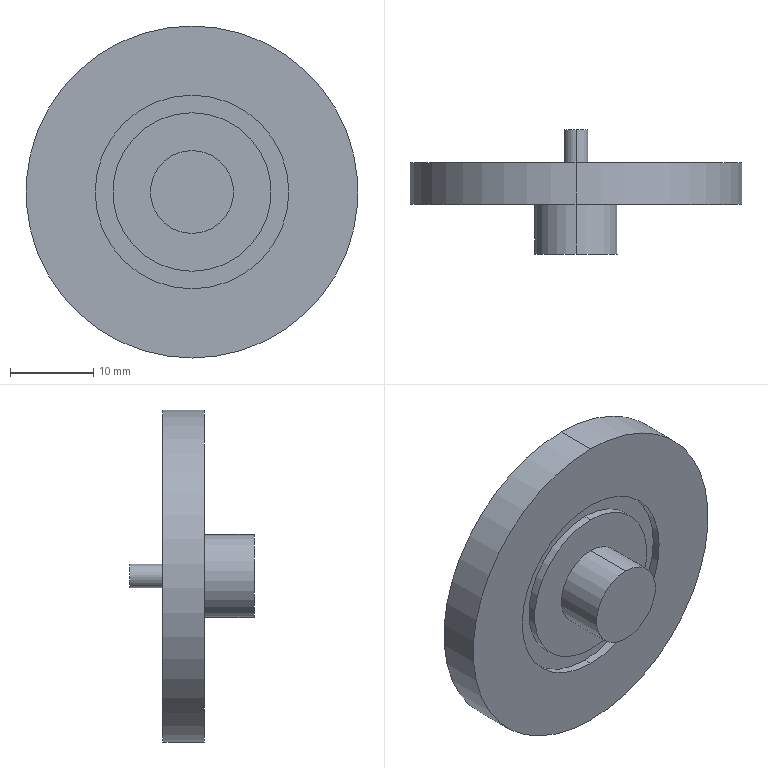Part | SolidWorks | features ICE 5, Extrusion 1 | 1 solid | 28 faces | box 40 x 15 x 40 mm | volume 6357 mm3 | cylinder 18 | plane 10 | commonest cylinder face diameters 2.85 x2 10 x2 16.818 x2 19.091 x2 20.068 x2 23.339 x2
STEP:
#1=CARTESIAN_POINT('',(0.,9.,1.425));
#2=VERTEX_POINT('',#1);
#3=CARTESIAN_POINT('',(0.,9.,-1.425));
#4=VERTEX_POINT('',#3);
#5=CARTESIAN_POINT('',(0.,9.,0.));
#6=DIRECTION('',(0.,1.,0.));
#7=DIRECTION('',(0.,0.,1.));
#8=AXIS2_PLACEMENT_3D('',#5,#6,#7);
#9=CIRCLE('',#8,1.425);
#10=EDGE_CURVE('',#2,#4,#9,.T.);
#11=ORIENTED_EDGE('',*,*,#10,.F.);
#12=CARTESIAN_POINT('',(0.,5.,1.425));
#13=VERTEX_POINT('',#12);
#14=CARTESIAN_POINT('',(0.,9.,1.425));
#15=DIRECTION('',(0.,-1.,0.));
#16=VECTOR('',#15,1000.);
#17=LINE('',#14,#16);
#18=EDGE_CURVE('',#2,#13,#17,.T.);
#19=ORIENTED_EDGE('',*,*,#18,.T.);
#20=CARTESIAN_POINT('',(0.,5.,-1.425));
#21=VERTEX_POINT('',#20);
#22=CARTESIAN_POINT('',(0.,5.,0.));
#23=DIRECTION('',(0.,1.,0.));
#24=DIRECTION('',(0.,0.,1.));
#25=AXIS2_PLACEMENT_3D('',#22,#23,#24);
#26=CIRCLE('',#25,1.425);
#27=EDGE_CURVE('',#13,#21,#26,.T.);
#28=ORIENTED_EDGE('',*,*,#27,.T.);
#29=CARTESIAN_POINT('',(0.,9.,-1.425));
#30=DIRECTION('',(0.,-1.,0.));
#31=VECTOR('',#30,1000.);
#32=LINE('',#29,#31);
#33=EDGE_CURVE('',#4,#21,#32,.T.);
#34=ORIENTED_EDGE('',*,*,#33,.F.);
#35=EDGE_LOOP('',(#11,#19,#28,#34));
#36=FACE_OUTER_BOUND('',#35,.T.);
#37=CARTESIAN_POINT('',(0.,9.,0.));
#38=DIRECTION('',(0.,-1.,0.));
#39=DIRECTION('',(0.,0.,-1.));
#40=AXIS2_PLACEMENT_3D('',#37,#38,#39);
#41=CYLINDRICAL_SURFACE('',#40,1.425);
#42=ADVANCED_FACE('',(#36),#41,.T.);
#43=CARTESIAN_POINT('',(0.,4.,8.409));
#44=VERTEX_POINT('',#43);
#45=CARTESIAN_POINT('',(0.,4.,-8.409));
#46=VERTEX_POINT('',#45);
#47=CARTESIAN_POINT('',(0.,4.,0.));
#48=DIRECTION('',(0.,1.,0.));
#49=DIRECTION('',(0.,0.,1.));
#50=AXIS2_PLACEMENT_3D('',#47,#48,#49);
#51=CIRCLE('',#50,8.409);
#52=EDGE_CURVE('',#44,#46,#51,.T.);
#53=ORIENTED_EDGE('',*,*,#52,.T.);
#54=CARTESIAN_POINT('',(0.,5.,-8.409));
#55=VERTEX_POINT('',#54);
#56=CARTESIAN_POINT('',(0.,4.,-8.409));
#57=DIRECTION('',(0.,1.,0.));
#58=VECTOR('',#57,1000.);
#59=LINE('',#56,#58);
#60=EDGE_CURVE('',#46,#55,#59,.T.);
#61=ORIENTED_EDGE('',*,*,#60,.T.);
#62=CARTESIAN_POINT('',(0.,5.,8.409));
#63=VERTEX_POINT('',#62);
#64=CARTESIAN_POINT('',(0.,5.,0.));
#65=DIRECTION('',(0.,1.,0.));
#66=DIRECTION('',(0.,0.,1.));
#67=AXIS2_PLACEMENT_3D('',#64,#65,#66);
#68=CIRCLE('',#67,8.409);
#69=EDGE_CURVE('',#63,#55,#68,.T.);
#70=ORIENTED_EDGE('',*,*,#69,.F.);
#71=CARTESIAN_POINT('',(0.,4.,8.409));
#72=DIRECTION('',(0.,1.,0.));
#73=VECTOR('',#72,1000.);
#74=LINE('',#71,#73);
#75=EDGE_CURVE('',#44,#63,#74,.T.);
#76=ORIENTED_EDGE('',*,*,#75,.F.);
#77=EDGE_LOOP('',(#53,#61,#70,#76));
#78=FACE_OUTER_BOUND('',#77,.T.);
#79=CARTESIAN_POINT('',(0.,4.,0.));
#80=DIRECTION('',(0.,1.,0.));
#81=DIRECTION('',(0.,0.,1.));
#82=AXIS2_PLACEMENT_3D('',#79,#80,#81);
#83=CYLINDRICAL_SURFACE('',#82,8.409);
#84=ADVANCED_FACE('',(#78),#83,.T.);
#85=CARTESIAN_POINT('',(0.,4.,-10.034));
#86=VERTEX_POINT('',#85);
#87=CARTESIAN_POINT('',(0.,4.,10.034));
#88=VERTEX_POINT('',#87);
#89=CARTESIAN_POINT('',(0.,4.,0.));
#90=DIRECTION('',(0.,1.,0.));
#91=DIRECTION('',(0.,0.,1.));
#92=AXIS2_PLACEMENT_3D('',#89,#90,#91);
#93=CIRCLE('',#92,10.034);
#94=EDGE_CURVE('',#86,#88,#93,.T.);
#95=ORIENTED_EDGE('',*,*,#94,.F.);
#96=CARTESIAN_POINT('',(0.,5.,-10.034));
#97=VERTEX_POINT('',#96);
#98=CARTESIAN_POINT('',(0.,4.,-10.034));
#99=DIRECTION('',(0.,1.,0.));
#100=VECTOR('',#99,1000.);
#101=LINE('',#98,#100);
#102=EDGE_CURVE('',#86,#97,#101,.T.);
#103=ORIENTED_EDGE('',*,*,#102,.T.);
#104=CARTESIAN_POINT('',(0.,5.,10.034));
#105=VERTEX_POINT('',#104);
#106=CARTESIAN_POINT('',(0.,5.,0.));
#107=DIRECTION('',(0.,1.,0.));
#108=DIRECTION('',(0.,0.,1.));
#109=AXIS2_PLACEMENT_3D('',#106,#107,#108);
#110=CIRCLE('',#109,10.034);
#111=EDGE_CURVE('',#97,#105,#110,.T.);
#112=ORIENTED_EDGE('',*,*,#111,.T.);
#113=CARTESIAN_POINT('',(0.,4.,10.034));
#114=DIRECTION('',(0.,1.,0.));
#115=VECTOR('',#114,1000.);
#116=LINE('',#113,#115);
#117=EDGE_CURVE('',#88,#105,#116,.T.);
#118=ORIENTED_EDGE('',*,*,#117,.F.);
#119=EDGE_LOOP('',(#95,#103,#112,#118));
#120=FACE_OUTER_BOUND('',#119,.T.);
#121=CARTESIAN_POINT('',(0.,4.,0.));
#122=DIRECTION('',(0.,1.,0.));
#123=DIRECTION('',(0.,0.,1.));
#124=AXIS2_PLACEMENT_3D('',#121,#122,#123);
#125=CYLINDRICAL_SURFACE('',#124,10.034);
#126=ADVANCED_FACE('',(#120),#125,.F.);
#127=CARTESIAN_POINT('',(0.,4.,15.634));
#128=VERTEX_POINT('',#127);
#129=CARTESIAN_POINT('',(0.,4.,-15.634));
#130=VERTEX_POINT('',#129);
#131=CARTESIAN_POINT('',(0.,4.,0.));
#132=DIRECTION('',(0.,1.,0.));
#133=DIRECTION('',(0.,0.,1.));
#134=AXIS2_PLACEMENT_3D('',#131,#132,#133);
#135=CIRCLE('',#134,15.634);
#136=EDGE_CURVE('',#128,#130,#135,.T.);
#137=ORIENTED_EDGE('',*,*,#136,.T.);
#138=CARTESIAN_POINT('',(0.,5.,-15.634));
#139=VERTEX_POINT('',#138);
#140=CARTESIAN_POINT('',(0.,4.,-15.634));
#141=DIRECTION('',(0.,1.,0.));
#142=VECTOR('',#141,1000.);
#143=LINE('',#140,#142);
#144=EDGE_CURVE('',#130,#139,#143,.T.);
#145=ORIENTED_EDGE('',*,*,#144,.T.);
#146=CARTESIAN_POINT('',(0.,5.,15.634));
#147=VERTEX_POINT('',#146);
#148=CARTESIAN_POINT('',(0.,5.,0.));
#149=DIRECTION('',(0.,1.,0.));
#150=DIRECTION('',(0.,0.,1.));
#151=AXIS2_PLACEMENT_3D('',#148,#149,#150);
#152=CIRCLE('',#151,15.634);
#153=EDGE_CURVE('',#147,#139,#152,.T.);
#154=ORIENTED_EDGE('',*,*,#153,.F.);
#155=CARTESIAN_POINT('',(0.,4.,15.634));
#156=DIRECTION('',(0.,1.,0.));
#157=VECTOR('',#156,1000.);
#158=LINE('',#155,#157);
#159=EDGE_CURVE('',#128,#147,#158,.T.);
#160=ORIENTED_EDGE('',*,*,#159,.F.);
#161=EDGE_LOOP('',(#137,#145,#154,#160));
#162=FACE_OUTER_BOUND('',#161,.T.);
#163=CARTESIAN_POINT('',(0.,4.,0.));
#164=DIRECTION('',(0.,1.,0.));
#165=DIRECTION('',(0.,0.,1.));
#166=AXIS2_PLACEMENT_3D('',#163,#164,#165);
#167=CYLINDRICAL_SURFACE('',#166,15.634);
#168=ADVANCED_FACE('',(#162),#167,.T.);
#169=CARTESIAN_POINT('',(0.,4.,-17.435));
#170=VERTEX_POINT('',#169);
#171=CARTESIAN_POINT('',(0.,4.,17.435));
#172=VERTEX_POINT('',#171);
#173=CARTESIAN_POINT('',(0.,4.,0.));
#174=DIRECTION('',(0.,1.,0.));
#175=DIRECTION('',(0.,0.,1.));
#176=AXIS2_PLACEMENT_3D('',#173,#174,#175);
#177=CIRCLE('',#176,17.435);
#178=EDGE_CURVE('',#170,#172,#177,.T.);
#179=ORIENTED_EDGE('',*,*,#178,.F.);
#180=CARTESIAN_POINT('',(0.,5.,-17.435));
#181=VERTEX_POINT('',#180);
#182=CARTESIAN_POINT('',(0.,4.,-17.435));
#183=DIRECTION('',(0.,1.,0.));
#184=VECTOR('',#183,1000.);
#185=LINE('',#182,#184);
#186=EDGE_CURVE('',#170,#181,#185,.T.);
#187=ORIENTED_EDGE('',*,*,#186,.T.);
#188=CARTESIAN_POINT('',(0.,5.,17.435));
#189=VERTEX_POINT('',#188);
#190=CARTESIAN_POINT('',(0.,5.,0.));
#191=DIRECTION('',(0.,1.,0.));
#192=DIRECTION('',(0.,0.,1.));
#193=AXIS2_PLACEMENT_3D('',#190,#191,#192);
#194=CIRCLE('',#193,17.435);
#195=EDGE_CURVE('',#181,#189,#194,.T.);
#196=ORIENTED_EDGE('',*,*,#195,.T.);
#197=CARTESIAN_POINT('',(0.,4.,17.435));
#198=DIRECTION('',(0.,1.,0.));
#199=VECTOR('',#198,1000.);
#200=LINE('',#197,#199);
#201=EDGE_CURVE('',#172,#189,#200,.T.);
#202=ORIENTED_EDGE('',*,*,#201,.F.);
#203=EDGE_LOOP('',(#179,#187,#196,#202));
#204=FACE_OUTER_BOUND('',#203,.T.);
#205=CARTESIAN_POINT('',(0.,4.,0.));
#206=DIRECTION('',(0.,1.,0.));
#207=DIRECTION('',(0.,0.,1.));
#208=AXIS2_PLACEMENT_3D('',#205,#206,#207);
#209=CYLINDRICAL_SURFACE('',#208,17.435);
#210=ADVANCED_FACE('',(#204),#209,.F.);
#211=CARTESIAN_POINT('',(0.,-6.,-5.));
#212=VERTEX_POINT('',#211);
#213=CARTESIAN_POINT('',(0.,-6.,5.));
#214=VERTEX_POINT('',#213);
#215=CARTESIAN_POINT('',(0.,-6.,0.));
#216=DIRECTION('',(0.,-1.,0.));
#217=DIRECTION('',(0.,0.,-1.));
#218=AXIS2_PLACEMENT_3D('',#215,#216,#217);
#219=CIRCLE('',#218,5.);
#220=EDGE_CURVE('',#212,#214,#219,.T.);
#221=ORIENTED_EDGE('',*,*,#220,.F.);
#222=CARTESIAN_POINT('',(0.,0.,-5.));
#223=VERTEX_POINT('',#222);
#224=CARTESIAN_POINT('',(0.,-6.,-5.));
#225=DIRECTION('',(0.,1.,0.));
#226=VECTOR('',#225,1000.);
#227=LINE('',#224,#226);
#228=EDGE_CURVE('',#212,#223,#227,.T.);
#229=ORIENTED_EDGE('',*,*,#228,.T.);
#230=CARTESIAN_POINT('',(0.,0.,5.));
#231=VERTEX_POINT('',#230);
#232=CARTESIAN_POINT('',(0.,0.,0.));
#233=DIRECTION('',(0.,-1.,0.));
#234=DIRECTION('',(0.,0.,-1.));
#235=AXIS2_PLACEMENT_3D('',#232,#233,#234);
#236=CIRCLE('',#235,5.);
#237=EDGE_CURVE('',#223,#231,#236,.T.);
#238=ORIENTED_EDGE('',*,*,#237,.T.);
#239=CARTESIAN_POINT('',(0.,-6.,5.));
#240=DIRECTION('',(0.,1.,0.));
#241=VECTOR('',#240,1000.);
#242=LINE('',#239,#241);
#243=EDGE_CURVE('',#214,#231,#242,.T.);
#244=ORIENTED_EDGE('',*,*,#243,.F.);
#245=EDGE_LOOP('',(#221,#229,#238,#244));
#246=FACE_OUTER_BOUND('',#245,.T.);
#247=CARTESIAN_POINT('',(0.,-6.,0.));
#248=DIRECTION('',(0.,1.,0.));
#249=DIRECTION('',(0.,0.,1.));
#250=AXIS2_PLACEMENT_3D('',#247,#248,#249);
#251=CYLINDRICAL_SURFACE('',#250,5.);
#252=ADVANCED_FACE('',(#246),#251,.T.);
#253=CARTESIAN_POINT('',(0.,1.,-9.545));
#254=VERTEX_POINT('',#253);
#255=CARTESIAN_POINT('',(0.,1.,9.545));
#256=VERTEX_POINT('',#255);
#257=CARTESIAN_POINT('',(0.,1.,0.));
#258=DIRECTION('',(0.,-1.,0.));
#259=DIRECTION('',(0.,0.,-1.));
#260=AXIS2_PLACEMENT_3D('',#257,#258,#259);
#261=CIRCLE('',#260,9.545);
#262=EDGE_CURVE('',#254,#256,#261,.T.);
#263=ORIENTED_EDGE('',*,*,#262,.T.);
#264=CARTESIAN_POINT('',(0.,0.,9.545));
#265=VERTEX_POINT('',#264);
#266=CARTESIAN_POINT('',(0.,1.,9.545));
#267=DIRECTION('',(0.,-1.,0.));
#268=VECTOR('',#267,1000.);
#269=LINE('',#266,#268);
#270=EDGE_CURVE('',#256,#265,#269,.T.);
#271=ORIENTED_EDGE('',*,*,#270,.T.);
#272=CARTESIAN_POINT('',(0.,0.,-9.545));
#273=VERTEX_POINT('',#272);
#274=CARTESIAN_POINT('',(0.,0.,0.));
#275=DIRECTION('',(0.,-1.,0.));
#276=DIRECTION('',(0.,0.,-1.));
#277=AXIS2_PLACEMENT_3D('',#274,#275,#276);
#278=CIRCLE('',#277,9.545);
#279=EDGE_CURVE('',#273,#265,#278,.T.);
#280=ORIENTED_EDGE('',*,*,#279,.F.);
#281=CARTESIAN_POINT('',(0.,1.,-9.545));
#282=DIRECTION('',(0.,-1.,0.));
#283=VECTOR('',#282,1000.);
#284=LINE('',#281,#283);
#285=EDGE_CURVE('',#254,#273,#284,.T.);
#286=ORIENTED_EDGE('',*,*,#285,.F.);
#287=EDGE_LOOP('',(#263,#271,#280,#286));
#288=FACE_OUTER_BOUND('',#287,.T.);
#289=CARTESIAN_POINT('',(0.,1.,0.));
#290=DIRECTION('',(0.,-1.,0.));
#291=DIRECTION('',(0.,0.,-1.));
#292=AXIS2_PLACEMENT_3D('',#289,#290,#291);
#293=CYLINDRICAL_SURFACE('',#292,9.545);
#294=ADVANCED_FACE('',(#288),#293,.T.);
#295=CARTESIAN_POINT('',(0.,1.,11.669));
#296=VERTEX_POINT('',#295);
#297=CARTESIAN_POINT('',(0.,1.,-11.669));
#298=VERTEX_POINT('',#297);
#299=CARTESIAN_POINT('',(0.,1.,0.));
#300=DIRECTION('',(0.,-1.,0.));
#301=DIRECTION('',(0.,0.,-1.));
#302=AXIS2_PLACEMENT_3D('',#299,#300,#301);
#303=CIRCLE('',#302,11.669);
#304=EDGE_CURVE('',#296,#298,#303,.T.);
#305=ORIENTED_EDGE('',*,*,#304,.F.);
#306=CARTESIAN_POINT('',(0.,0.,11.669));
#307=VERTEX_POINT('',#306);
#308=CARTESIAN_POINT('',(0.,1.,11.669));
#309=DIRECTION('',(0.,-1.,0.));
#310=VECTOR('',#309,1000.);
#311=LINE('',#308,#310);
#312=EDGE_CURVE('',#296,#307,#311,.T.);
#313=ORIENTED_EDGE('',*,*,#312,.T.);
#314=CARTESIAN_POINT('',(0.,0.,-11.669));
#315=VERTEX_POINT('',#314);
#316=CARTESIAN_POINT('',(0.,0.,0.));
#317=DIRECTION('',(0.,-1.,0.));
#318=DIRECTION('',(0.,0.,-1.));
#319=AXIS2_PLACEMENT_3D('',#316,#317,#318);
#320=CIRCLE('',#319,11.669);
#321=EDGE_CURVE('',#307,#315,#320,.T.);
#322=ORIENTED_EDGE('',*,*,#321,.T.);
#323=CARTESIAN_POINT('',(0.,1.,-11.669));
#324=DIRECTION('',(0.,-1.,0.));
#325=VECTOR('',#324,1000.);
#326=LINE('',#323,#325);
#327=EDGE_CURVE('',#298,#315,#326,.T.);
#328=ORIENTED_EDGE('',*,*,#327,.F.);
#329=EDGE_LOOP('',(#305,#313,#322,#328));
#330=FACE_OUTER_BOUND('',#329,.T.);
#331=CARTESIAN_POINT('',(0.,1.,0.));
#332=DIRECTION('',(0.,-1.,0.));
#333=DIRECTION('',(0.,0.,-1.));
#334=AXIS2_PLACEMENT_3D('',#331,#332,#333);
#335=CYLINDRICAL_SURFACE('',#334,11.669);
#336=ADVANCED_FACE('',(#330),#335,.F.);
#337=CARTESIAN_POINT('',(0.,5.,20.));
#338=VERTEX_POINT('',#337);
#339=CARTESIAN_POINT('',(0.,5.,-20.));
#340=VERTEX_POINT('',#339);
#341=CARTESIAN_POINT('',(0.,5.,0.));
#342=DIRECTION('',(0.,1.,0.));
#343=DIRECTION('',(0.,0.,1.));
#344=AXIS2_PLACEMENT_3D('',#341,#342,#343);
#345=CIRCLE('',#344,20.);
#346=EDGE_CURVE('',#338,#340,#345,.T.);
#347=ORIENTED_EDGE('',*,*,#346,.F.);
#348=CARTESIAN_POINT('',(0.,0.,20.));
#349=VERTEX_POINT('',#348);
#350=CARTESIAN_POINT('',(0.,5.,20.));
#351=DIRECTION('',(0.,-1.,0.));
#352=VECTOR('',#351,1000.);
#353=LINE('',#350,#352);
#354=EDGE_CURVE('',#338,#349,#353,.T.);
#355=ORIENTED_EDGE('',*,*,#354,.T.);
#356=CARTESIAN_POINT('',(0.,0.,-20.));
#357=VERTEX_POINT('',#356);
#358=CARTESIAN_POINT('',(0.,0.,0.));
#359=DIRECTION('',(0.,1.,0.));
#360=DIRECTION('',(0.,0.,1.));
#361=AXIS2_PLACEMENT_3D('',#358,#359,#360);
#362=CIRCLE('',#361,20.);
#363=EDGE_CURVE('',#349,#357,#362,.T.);
#364=ORIENTED_EDGE('',*,*,#363,.T.);
#365=CARTESIAN_POINT('',(0.,5.,-20.));
#366=DIRECTION('',(0.,-1.,0.));
#367=VECTOR('',#366,1000.);
#368=LINE('',#365,#367);
#369=EDGE_CURVE('',#340,#357,#368,.T.);
#370=ORIENTED_EDGE('',*,*,#369,.F.);
#371=EDGE_LOOP('',(#347,#355,#364,#370));
#372=FACE_OUTER_BOUND('',#371,.T.);
#373=CARTESIAN_POINT('',(0.,5.,0.));
#374=DIRECTION('',(0.,-1.,0.));
#375=DIRECTION('',(0.,0.,-1.));
#376=AXIS2_PLACEMENT_3D('',#373,#374,#375);
#377=CYLINDRICAL_SURFACE('',#376,20.);
#378=ADVANCED_FACE('',(#372),#377,.T.);
#379=ORIENTED_EDGE('',*,*,#354,.F.);
#380=CARTESIAN_POINT('',(0.,5.,0.));
#381=DIRECTION('',(0.,1.,0.));
#382=DIRECTION('',(0.,0.,1.));
#383=AXIS2_PLACEMENT_3D('',#380,#381,#382);
#384=CIRCLE('',#383,20.);
#385=EDGE_CURVE('',#340,#338,#384,.T.);
#386=ORIENTED_EDGE('',*,*,#385,.F.);
#387=ORIENTED_EDGE('',*,*,#369,.T.);
#388=CARTESIAN_POINT('',(0.,0.,0.));
#389=DIRECTION('',(0.,1.,0.));
#390=DIRECTION('',(0.,0.,1.));
#391=AXIS2_PLACEMENT_3D('',#388,#389,#390);
#392=CIRCLE('',#391,20.);
#393=EDGE_CURVE('',#357,#349,#392,.T.);
#394=ORIENTED_EDGE('',*,*,#393,.T.);
#395=EDGE_LOOP('',(#379,#386,#387,#394));
#396=FACE_OUTER_BOUND('',#395,.T.);
#397=CARTESIAN_POINT('',(0.,5.,0.));
#398=DIRECTION('',(0.,-1.,0.));
#399=DIRECTION('',(0.,0.,-1.));
#400=AXIS2_PLACEMENT_3D('',#397,#398,#399);
#401=CYLINDRICAL_SURFACE('',#400,20.);
#402=ADVANCED_FACE('',(#396),#401,.T.);
#403=CARTESIAN_POINT('',(0.,5.,0.));
#404=DIRECTION('',(0.,1.,0.));
#405=DIRECTION('',(0.,0.,1.));
#406=AXIS2_PLACEMENT_3D('',#403,#404,#405);
#407=CIRCLE('',#406,17.435);
#408=EDGE_CURVE('',#189,#181,#407,.T.);
#409=ORIENTED_EDGE('',*,*,#408,.F.);
#410=ORIENTED_EDGE('',*,*,#195,.F.);
#411=EDGE_LOOP('',(#409,#410));
#412=FACE_BOUND('',#411,.T.);
#413=ORIENTED_EDGE('',*,*,#385,.T.);
#414=ORIENTED_EDGE('',*,*,#346,.T.);
#415=EDGE_LOOP('',(#413,#414));
#416=FACE_OUTER_BOUND('',#415,.T.);
#417=CARTESIAN_POINT('',(0.,5.,0.));
#418=DIRECTION('',(0.,1.,0.));
#419=DIRECTION('',(0.,0.,1.));
#420=AXIS2_PLACEMENT_3D('',#417,#418,#419);
#421=PLANE('',#420);
#422=ADVANCED_FACE('',(#412,#416),#421,.T.);
#423=CARTESIAN_POINT('',(0.,0.,0.));
#424=DIRECTION('',(0.,-1.,0.));
#425=DIRECTION('',(0.,0.,-1.));
#426=AXIS2_PLACEMENT_3D('',#423,#424,#425);
#427=CIRCLE('',#426,11.669);
#428=EDGE_CURVE('',#315,#307,#427,.T.);
#429=ORIENTED_EDGE('',*,*,#428,.F.);
#430=ORIENTED_EDGE('',*,*,#321,.F.);
#431=EDGE_LOOP('',(#429,#430));
#432=FACE_BOUND('',#431,.T.);
#433=ORIENTED_EDGE('',*,*,#393,.F.);
#434=ORIENTED_EDGE('',*,*,#363,.F.);
#435=EDGE_LOOP('',(#433,#434));
#436=FACE_OUTER_BOUND('',#435,.T.);
#437=CARTESIAN_POINT('',(0.,0.,0.));
#438=DIRECTION('',(0.,1.,0.));
#439=DIRECTION('',(0.,0.,1.));
#440=AXIS2_PLACEMENT_3D('',#437,#438,#439);
#441=PLANE('',#440);
#442=ADVANCED_FACE('',(#432,#436),#441,.F.);
#443=ORIENTED_EDGE('',*,*,#312,.F.);
#444=CARTESIAN_POINT('',(0.,1.,0.));
#445=DIRECTION('',(0.,-1.,0.));
#446=DIRECTION('',(0.,0.,-1.));
#447=AXIS2_PLACEMENT_3D('',#444,#445,#446);
#448=CIRCLE('',#447,11.669);
#449=EDGE_CURVE('',#298,#296,#448,.T.);
#450=ORIENTED_EDGE('',*,*,#449,.F.);
#451=ORIENTED_EDGE('',*,*,#327,.T.);
#452=ORIENTED_EDGE('',*,*,#428,.T.);
#453=EDGE_LOOP('',(#443,#450,#451,#452));
#454=FACE_OUTER_BOUND('',#453,.T.);
#455=CARTESIAN_POINT('',(0.,1.,0.));
#456=DIRECTION('',(0.,-1.,0.));
#457=DIRECTION('',(0.,0.,-1.));
#458=AXIS2_PLACEMENT_3D('',#455,#456,#457);
#459=CYLINDRICAL_SURFACE('',#458,11.669);
#460=ADVANCED_FACE('',(#454),#459,.F.);
#461=ORIENTED_EDGE('',*,*,#262,.F.);
#462=CARTESIAN_POINT('',(0.,1.,0.));
#463=DIRECTION('',(0.,-1.,0.));
#464=DIRECTION('',(0.,0.,-1.));
#465=AXIS2_PLACEMENT_3D('',#462,#463,#464);
#466=CIRCLE('',#465,9.545);
#467=EDGE_CURVE('',#256,#254,#466,.T.);
#468=ORIENTED_EDGE('',*,*,#467,.F.);
#469=EDGE_LOOP('',(#461,#468));
#470=FACE_BOUND('',#469,.T.);
#471=ORIENTED_EDGE('',*,*,#449,.T.);
#472=ORIENTED_EDGE('',*,*,#304,.T.);
#473=EDGE_LOOP('',(#471,#472));
#474=FACE_OUTER_BOUND('',#473,.T.);
#475=CARTESIAN_POINT('',(0.,1.,0.));
#476=DIRECTION('',(0.,-1.,0.));
#477=DIRECTION('',(0.,0.,-1.));
#478=AXIS2_PLACEMENT_3D('',#475,#476,#477);
#479=PLANE('',#478);
#480=ADVANCED_FACE('',(#470,#474),#479,.T.);
#481=ORIENTED_EDGE('',*,*,#270,.F.);
#482=ORIENTED_EDGE('',*,*,#467,.T.);
#483=ORIENTED_EDGE('',*,*,#285,.T.);
#484=CARTESIAN_POINT('',(0.,0.,0.));
#485=DIRECTION('',(0.,-1.,0.));
#486=DIRECTION('',(0.,0.,-1.));
#487=AXIS2_PLACEMENT_3D('',#484,#485,#486);
#488=CIRCLE('',#487,9.545);
#489=EDGE_CURVE('',#265,#273,#488,.T.);
#490=ORIENTED_EDGE('',*,*,#489,.F.);
#491=EDGE_LOOP('',(#481,#482,#483,#490));
#492=FACE_OUTER_BOUND('',#491,.T.);
#493=CARTESIAN_POINT('',(0.,1.,0.));
#494=DIRECTION('',(0.,-1.,0.));
#495=DIRECTION('',(0.,0.,-1.));
#496=AXIS2_PLACEMENT_3D('',#493,#494,#495);
#497=CYLINDRICAL_SURFACE('',#496,9.545);
#498=ADVANCED_FACE('',(#492),#497,.T.);
#499=CARTESIAN_POINT('',(0.,-6.,0.));
#500=DIRECTION('',(0.,-1.,0.));
#501=DIRECTION('',(0.,0.,-1.));
#502=AXIS2_PLACEMENT_3D('',#499,#500,#501);
#503=CIRCLE('',#502,5.);
#504=EDGE_CURVE('',#214,#212,#503,.T.);
#505=ORIENTED_EDGE('',*,*,#504,.T.);
#506=ORIENTED_EDGE('',*,*,#220,.T.);
#507=EDGE_LOOP('',(#505,#506));
#508=FACE_OUTER_BOUND('',#507,.T.);
#509=CARTESIAN_POINT('',(0.,-6.,0.));
#510=DIRECTION('',(0.,-1.,0.));
#511=DIRECTION('',(0.,0.,-1.));
#512=AXIS2_PLACEMENT_3D('',#509,#510,#511);
#513=PLANE('',#512);
#514=ADVANCED_FACE('',(#508),#513,.T.);
#515=ORIENTED_EDGE('',*,*,#228,.F.);
#516=ORIENTED_EDGE('',*,*,#504,.F.);
#517=ORIENTED_EDGE('',*,*,#243,.T.);
#518=CARTESIAN_POINT('',(0.,0.,0.));
#519=DIRECTION('',(0.,-1.,0.));
#520=DIRECTION('',(0.,0.,-1.));
#521=AXIS2_PLACEMENT_3D('',#518,#519,#520);
#522=CIRCLE('',#521,5.);
#523=EDGE_CURVE('',#231,#223,#522,.T.);
#524=ORIENTED_EDGE('',*,*,#523,.T.);
#525=EDGE_LOOP('',(#515,#516,#517,#524));
#526=FACE_OUTER_BOUND('',#525,.T.);
#527=CARTESIAN_POINT('',(0.,-6.,0.));
#528=DIRECTION('',(0.,1.,0.));
#529=DIRECTION('',(0.,0.,1.));
#530=AXIS2_PLACEMENT_3D('',#527,#528,#529);
#531=CYLINDRICAL_SURFACE('',#530,5.);
#532=ADVANCED_FACE('',(#526),#531,.T.);
#533=ORIENTED_EDGE('',*,*,#523,.F.);
#534=ORIENTED_EDGE('',*,*,#237,.F.);
#535=EDGE_LOOP('',(#533,#534));
#536=FACE_BOUND('',#535,.T.);
#537=ORIENTED_EDGE('',*,*,#279,.T.);
#538=ORIENTED_EDGE('',*,*,#489,.T.);
#539=EDGE_LOOP('',(#537,#538));
#540=FACE_OUTER_BOUND('',#539,.T.);
#541=CARTESIAN_POINT('',(0.,0.,0.));
#542=DIRECTION('',(0.,1.,0.));
#543=DIRECTION('',(0.,0.,1.));
#544=AXIS2_PLACEMENT_3D('',#541,#542,#543);
#545=PLANE('',#544);
#546=ADVANCED_FACE('',(#536,#540),#545,.F.);
#547=ORIENTED_EDGE('',*,*,#186,.F.);
#548=CARTESIAN_POINT('',(0.,4.,0.));
#549=DIRECTION('',(0.,1.,0.));
#550=DIRECTION('',(0.,0.,1.));
#551=AXIS2_PLACEMENT_3D('',#548,#549,#550);
#552=CIRCLE('',#551,17.435);
#553=EDGE_CURVE('',#172,#170,#552,.T.);
#554=ORIENTED_EDGE('',*,*,#553,.F.);
#555=ORIENTED_EDGE('',*,*,#201,.T.);
#556=ORIENTED_EDGE('',*,*,#408,.T.);
#557=EDGE_LOOP('',(#547,#554,#555,#556));
#558=FACE_OUTER_BOUND('',#557,.T.);
#559=CARTESIAN_POINT('',(0.,4.,0.));
#560=DIRECTION('',(0.,1.,0.));
#561=DIRECTION('',(0.,0.,1.));
#562=AXIS2_PLACEMENT_3D('',#559,#560,#561);
#563=CYLINDRICAL_SURFACE('',#562,17.435);
#564=ADVANCED_FACE('',(#558),#563,.F.);
#565=ORIENTED_EDGE('',*,*,#136,.F.);
#566=CARTESIAN_POINT('',(0.,4.,0.));
#567=DIRECTION('',(0.,1.,0.));
#568=DIRECTION('',(0.,0.,1.));
#569=AXIS2_PLACEMENT_3D('',#566,#567,#568);
#570=CIRCLE('',#569,15.634);
#571=EDGE_CURVE('',#130,#128,#570,.T.);
#572=ORIENTED_EDGE('',*,*,#571,.F.);
#573=EDGE_LOOP('',(#565,#572));
#574=FACE_BOUND('',#573,.T.);
#575=ORIENTED_EDGE('',*,*,#553,.T.);
#576=ORIENTED_EDGE('',*,*,#178,.T.);
#577=EDGE_LOOP('',(#575,#576));
#578=FACE_OUTER_BOUND('',#577,.T.);
#579=CARTESIAN_POINT('',(0.,4.,0.));
#580=DIRECTION('',(0.,1.,0.));
#581=DIRECTION('',(0.,0.,1.));
#582=AXIS2_PLACEMENT_3D('',#579,#580,#581);
#583=PLANE('',#582);
#584=ADVANCED_FACE('',(#574,#578),#583,.T.);
#585=ORIENTED_EDGE('',*,*,#144,.F.);
#586=ORIENTED_EDGE('',*,*,#571,.T.);
#587=ORIENTED_EDGE('',*,*,#159,.T.);
#588=CARTESIAN_POINT('',(0.,5.,0.));
#589=DIRECTION('',(0.,1.,0.));
#590=DIRECTION('',(0.,0.,1.));
#591=AXIS2_PLACEMENT_3D('',#588,#589,#590);
#592=CIRCLE('',#591,15.634);
#593=EDGE_CURVE('',#139,#147,#592,.T.);
#594=ORIENTED_EDGE('',*,*,#593,.F.);
#595=EDGE_LOOP('',(#585,#586,#587,#594));
#596=FACE_OUTER_BOUND('',#595,.T.);
#597=CARTESIAN_POINT('',(0.,4.,0.));
#598=DIRECTION('',(0.,1.,0.));
#599=DIRECTION('',(0.,0.,1.));
#600=AXIS2_PLACEMENT_3D('',#597,#598,#599);
#601=CYLINDRICAL_SURFACE('',#600,15.634);
#602=ADVANCED_FACE('',(#596),#601,.T.);
#603=CARTESIAN_POINT('',(0.,5.,0.));
#604=DIRECTION('',(0.,1.,0.));
#605=DIRECTION('',(0.,0.,1.));
#606=AXIS2_PLACEMENT_3D('',#603,#604,#605);
#607=CIRCLE('',#606,10.034);
#608=EDGE_CURVE('',#105,#97,#607,.T.);
#609=ORIENTED_EDGE('',*,*,#608,.F.);
#610=ORIENTED_EDGE('',*,*,#111,.F.);
#611=EDGE_LOOP('',(#609,#610));
#612=FACE_BOUND('',#611,.T.);
#613=ORIENTED_EDGE('',*,*,#153,.T.);
#614=ORIENTED_EDGE('',*,*,#593,.T.);
#615=EDGE_LOOP('',(#613,#614));
#616=FACE_OUTER_BOUND('',#615,.T.);
#617=CARTESIAN_POINT('',(0.,5.,0.));
#618=DIRECTION('',(0.,1.,0.));
#619=DIRECTION('',(0.,0.,1.));
#620=AXIS2_PLACEMENT_3D('',#617,#618,#619);
#621=PLANE('',#620);
#622=ADVANCED_FACE('',(#612,#616),#621,.T.);
#623=ORIENTED_EDGE('',*,*,#102,.F.);
#624=CARTESIAN_POINT('',(0.,4.,0.));
#625=DIRECTION('',(0.,1.,0.));
#626=DIRECTION('',(0.,0.,1.));
#627=AXIS2_PLACEMENT_3D('',#624,#625,#626);
#628=CIRCLE('',#627,10.034);
#629=EDGE_CURVE('',#88,#86,#628,.T.);
#630=ORIENTED_EDGE('',*,*,#629,.F.);
#631=ORIENTED_EDGE('',*,*,#117,.T.);
#632=ORIENTED_EDGE('',*,*,#608,.T.);
#633=EDGE_LOOP('',(#623,#630,#631,#632));
#634=FACE_OUTER_BOUND('',#633,.T.);
#635=CARTESIAN_POINT('',(0.,4.,0.));
#636=DIRECTION('',(0.,1.,0.));
#637=DIRECTION('',(0.,0.,1.));
#638=AXIS2_PLACEMENT_3D('',#635,#636,#637);
#639=CYLINDRICAL_SURFACE('',#638,10.034);
#640=ADVANCED_FACE('',(#634),#639,.F.);
#641=ORIENTED_EDGE('',*,*,#52,.F.);
#642=CARTESIAN_POINT('',(0.,4.,0.));
#643=DIRECTION('',(0.,1.,0.));
#644=DIRECTION('',(0.,0.,1.));
#645=AXIS2_PLACEMENT_3D('',#642,#643,#644);
#646=CIRCLE('',#645,8.409);
#647=EDGE_CURVE('',#46,#44,#646,.T.);
#648=ORIENTED_EDGE('',*,*,#647,.F.);
#649=EDGE_LOOP('',(#641,#648));
#650=FACE_BOUND('',#649,.T.);
#651=ORIENTED_EDGE('',*,*,#629,.T.);
#652=ORIENTED_EDGE('',*,*,#94,.T.);
#653=EDGE_LOOP('',(#651,#652));
#654=FACE_OUTER_BOUND('',#653,.T.);
#655=CARTESIAN_POINT('',(0.,4.,0.));
#656=DIRECTION('',(0.,1.,0.));
#657=DIRECTION('',(0.,0.,1.));
#658=AXIS2_PLACEMENT_3D('',#655,#656,#657);
#659=PLANE('',#658);
#660=ADVANCED_FACE('',(#650,#654),#659,.T.);
#661=ORIENTED_EDGE('',*,*,#60,.F.);
#662=ORIENTED_EDGE('',*,*,#647,.T.);
#663=ORIENTED_EDGE('',*,*,#75,.T.);
#664=CARTESIAN_POINT('',(0.,5.,0.));
#665=DIRECTION('',(0.,1.,0.));
#666=DIRECTION('',(0.,0.,1.));
#667=AXIS2_PLACEMENT_3D('',#664,#665,#666);
#668=CIRCLE('',#667,8.409);
#669=EDGE_CURVE('',#55,#63,#668,.T.);
#670=ORIENTED_EDGE('',*,*,#669,.F.);
#671=EDGE_LOOP('',(#661,#662,#663,#670));
#672=FACE_OUTER_BOUND('',#671,.T.);
#673=CARTESIAN_POINT('',(0.,4.,0.));
#674=DIRECTION('',(0.,1.,0.));
#675=DIRECTION('',(0.,0.,1.));
#676=AXIS2_PLACEMENT_3D('',#673,#674,#675);
#677=CYLINDRICAL_SURFACE('',#676,8.409);
#678=ADVANCED_FACE('',(#672),#677,.T.);
#679=CARTESIAN_POINT('',(0.,9.,0.));
#680=DIRECTION('',(0.,1.,0.));
#681=DIRECTION('',(0.,0.,1.));
#682=AXIS2_PLACEMENT_3D('',#679,#680,#681);
#683=CIRCLE('',#682,1.425);
#684=EDGE_CURVE('',#4,#2,#683,.T.);
#685=ORIENTED_EDGE('',*,*,#684,.T.);
#686=ORIENTED_EDGE('',*,*,#10,.T.);
#687=EDGE_LOOP('',(#685,#686));
#688=FACE_OUTER_BOUND('',#687,.T.);
#689=CARTESIAN_POINT('',(0.,9.,0.));
#690=DIRECTION('',(0.,1.,0.));
#691=DIRECTION('',(0.,0.,1.));
#692=AXIS2_PLACEMENT_3D('',#689,#690,#691);
#693=PLANE('',#692);
#694=ADVANCED_FACE('',(#688),#693,.T.);
#695=ORIENTED_EDGE('',*,*,#18,.F.);
#696=ORIENTED_EDGE('',*,*,#684,.F.);
#697=ORIENTED_EDGE('',*,*,#33,.T.);
#698=CARTESIAN_POINT('',(0.,5.,0.));
#699=DIRECTION('',(0.,1.,0.));
#700=DIRECTION('',(0.,0.,1.));
#701=AXIS2_PLACEMENT_3D('',#698,#699,#700);
#702=CIRCLE('',#701,1.425);
#703=EDGE_CURVE('',#21,#13,#702,.T.);
#704=ORIENTED_EDGE('',*,*,#703,.T.);
#705=EDGE_LOOP('',(#695,#696,#697,#704));
#706=FACE_OUTER_BOUND('',#705,.T.);
#707=CARTESIAN_POINT('',(0.,9.,0.));
#708=DIRECTION('',(0.,-1.,0.));
#709=DIRECTION('',(0.,0.,-1.));
#710=AXIS2_PLACEMENT_3D('',#707,#708,#709);
#711=CYLINDRICAL_SURFACE('',#710,1.425);
#712=ADVANCED_FACE('',(#706),#711,.T.);
#713=ORIENTED_EDGE('',*,*,#703,.F.);
#714=ORIENTED_EDGE('',*,*,#27,.F.);
#715=EDGE_LOOP('',(#713,#714));
#716=FACE_BOUND('',#715,.T.);
#717=ORIENTED_EDGE('',*,*,#69,.T.);
#718=ORIENTED_EDGE('',*,*,#669,.T.);
#719=EDGE_LOOP('',(#717,#718));
#720=FACE_OUTER_BOUND('',#719,.T.);
#721=CARTESIAN_POINT('',(0.,5.,0.));
#722=DIRECTION('',(0.,1.,0.));
#723=DIRECTION('',(0.,0.,1.));
#724=AXIS2_PLACEMENT_3D('',#721,#722,#723);
#725=PLANE('',#724);
#726=ADVANCED_FACE('',(#716,#720),#725,.T.);
#727=CLOSED_SHELL('',(#42,#84,#126,#168,#210,#252,#294,#336,#378,#402,#422,#442,#460,#480,#498,#514,#532,#546,#564,#584,#602,#622,#640,#660,#678,#694,#712,#726));
#728=MANIFOLD_SOLID_BREP('',#727);
#729=CARTESIAN_POINT('',(0.,0.,0.));
#730=DIRECTION('',(0.,0.,1.));
#731=DIRECTION('',(1.,0.,0.));
#732=AXIS2_PLACEMENT_3D('',#729,#730,#731);
#733=(LENGTH_UNIT()NAMED_UNIT(*)SI_UNIT(.MILLI.,.METRE.));
#734=UNCERTAINTY_MEASURE_WITH_UNIT(LENGTH_MEASURE(0.00001),#733,'','');
#735=(NAMED_UNIT(*)PLANE_ANGLE_UNIT()SI_UNIT($,.RADIAN.));
#736=(NAMED_UNIT(*)SI_UNIT($,.STERADIAN.)SOLID_ANGLE_UNIT());
#737=(GEOMETRIC_REPRESENTATION_CONTEXT(3)GLOBAL_UNCERTAINTY_ASSIGNED_CONTEXT((#734))GLOBAL_UNIT_ASSIGNED_CONTEXT((#733,#735,#736))REPRESENTATION_CONTEXT('',''));
#738=ADVANCED_BREP_SHAPE_REPRESENTATION('',(#728,#732),#737);